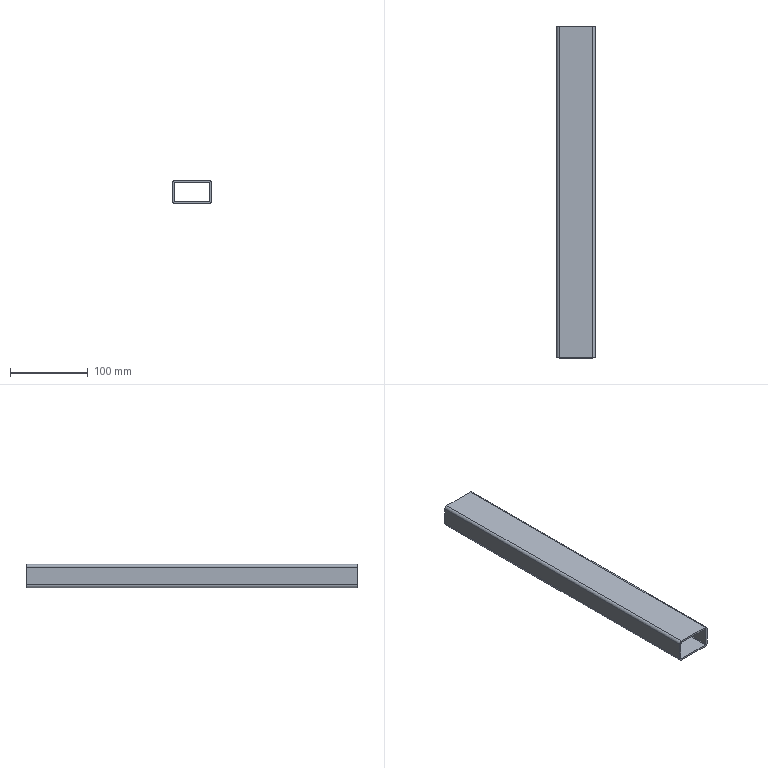Part | SolidWorks | features Extrusion 1 | 1 solid | 18 faces | box 50 x 428 x 30 mm | volume 144560 mm3 | plane 10 | cylinder 8 | commonest cylinder face diameters 2.3 x4 6.9 x4
STEP:
#1=CARTESIAN_POINT('',(25.,428.,-11.55));
#2=VERTEX_POINT('',#1);
#3=CARTESIAN_POINT('',(21.55,428.,-15.));
#4=VERTEX_POINT('',#3);
#5=CARTESIAN_POINT('',(21.55,428.,-11.55));
#6=DIRECTION('',(0.,1.,0.));
#7=DIRECTION('',(0.,0.,-1.));
#8=AXIS2_PLACEMENT_3D('',#5,#6,#7);
#9=CIRCLE('',#8,3.45);
#10=EDGE_CURVE('',#2,#4,#9,.T.);
#11=ORIENTED_EDGE('',*,*,#10,.T.);
#12=CARTESIAN_POINT('',(-21.55,428.,-15.));
#13=VERTEX_POINT('',#12);
#14=CARTESIAN_POINT('',(-21.55,428.,-15.));
#15=DIRECTION('',(-1.,0.,0.));
#16=VECTOR('',#15,1000.);
#17=LINE('',#14,#16);
#18=EDGE_CURVE('',#4,#13,#17,.T.);
#19=ORIENTED_EDGE('',*,*,#18,.T.);
#20=CARTESIAN_POINT('',(-25.,428.,-11.55));
#21=VERTEX_POINT('',#20);
#22=CARTESIAN_POINT('',(-21.55,428.,-11.55));
#23=DIRECTION('',(0.,1.,0.));
#24=DIRECTION('',(0.,0.,-1.));
#25=AXIS2_PLACEMENT_3D('',#22,#23,#24);
#26=CIRCLE('',#25,3.45);
#27=EDGE_CURVE('',#13,#21,#26,.T.);
#28=ORIENTED_EDGE('',*,*,#27,.T.);
#29=CARTESIAN_POINT('',(-25.,428.,11.55));
#30=VERTEX_POINT('',#29);
#31=CARTESIAN_POINT('',(-25.,428.,11.55));
#32=DIRECTION('',(0.,0.,1.));
#33=VECTOR('',#32,1000.);
#34=LINE('',#31,#33);
#35=EDGE_CURVE('',#21,#30,#34,.T.);
#36=ORIENTED_EDGE('',*,*,#35,.T.);
#37=CARTESIAN_POINT('',(-21.55,428.,15.));
#38=VERTEX_POINT('',#37);
#39=CARTESIAN_POINT('',(-21.55,428.,11.55));
#40=DIRECTION('',(0.,1.,0.));
#41=DIRECTION('',(0.,0.,-1.));
#42=AXIS2_PLACEMENT_3D('',#39,#40,#41);
#43=CIRCLE('',#42,3.45);
#44=EDGE_CURVE('',#30,#38,#43,.T.);
#45=ORIENTED_EDGE('',*,*,#44,.T.);
#46=CARTESIAN_POINT('',(21.55,428.,15.));
#47=VERTEX_POINT('',#46);
#48=CARTESIAN_POINT('',(-21.55,428.,15.));
#49=DIRECTION('',(1.,0.,0.));
#50=VECTOR('',#49,1000.);
#51=LINE('',#48,#50);
#52=EDGE_CURVE('',#38,#47,#51,.T.);
#53=ORIENTED_EDGE('',*,*,#52,.T.);
#54=CARTESIAN_POINT('',(25.,428.,11.55));
#55=VERTEX_POINT('',#54);
#56=CARTESIAN_POINT('',(21.55,428.,11.55));
#57=DIRECTION('',(0.,1.,0.));
#58=DIRECTION('',(0.,0.,1.));
#59=AXIS2_PLACEMENT_3D('',#56,#57,#58);
#60=CIRCLE('',#59,3.45);
#61=EDGE_CURVE('',#47,#55,#60,.T.);
#62=ORIENTED_EDGE('',*,*,#61,.T.);
#63=CARTESIAN_POINT('',(25.,428.,11.55));
#64=DIRECTION('',(0.,0.,-1.));
#65=VECTOR('',#64,1000.);
#66=LINE('',#63,#65);
#67=EDGE_CURVE('',#55,#2,#66,.T.);
#68=ORIENTED_EDGE('',*,*,#67,.T.);
#69=EDGE_LOOP('',(#11,#19,#28,#36,#45,#53,#62,#68));
#70=FACE_OUTER_BOUND('',#69,.T.);
#71=CARTESIAN_POINT('',(-22.7,428.,11.55));
#72=VERTEX_POINT('',#71);
#73=CARTESIAN_POINT('',(-21.55,428.,12.7));
#74=VERTEX_POINT('',#73);
#75=CARTESIAN_POINT('',(-21.55,428.,11.55));
#76=DIRECTION('',(0.,1.,0.));
#77=DIRECTION('',(0.,0.,-1.));
#78=AXIS2_PLACEMENT_3D('',#75,#76,#77);
#79=CIRCLE('',#78,1.15);
#80=EDGE_CURVE('',#72,#74,#79,.T.);
#81=ORIENTED_EDGE('',*,*,#80,.F.);
#82=CARTESIAN_POINT('',(-22.7,428.,-11.55));
#83=VERTEX_POINT('',#82);
#84=CARTESIAN_POINT('',(-22.7,428.,11.55));
#85=DIRECTION('',(0.,0.,1.));
#86=VECTOR('',#85,1000.);
#87=LINE('',#84,#86);
#88=EDGE_CURVE('',#83,#72,#87,.T.);
#89=ORIENTED_EDGE('',*,*,#88,.F.);
#90=CARTESIAN_POINT('',(-21.55,428.,-12.7));
#91=VERTEX_POINT('',#90);
#92=CARTESIAN_POINT('',(-21.55,428.,-11.55));
#93=DIRECTION('',(0.,1.,0.));
#94=DIRECTION('',(0.,0.,-1.));
#95=AXIS2_PLACEMENT_3D('',#92,#93,#94);
#96=CIRCLE('',#95,1.15);
#97=EDGE_CURVE('',#91,#83,#96,.T.);
#98=ORIENTED_EDGE('',*,*,#97,.F.);
#99=CARTESIAN_POINT('',(21.55,428.,-12.7));
#100=VERTEX_POINT('',#99);
#101=CARTESIAN_POINT('',(-21.55,428.,-12.7));
#102=DIRECTION('',(-1.,0.,0.));
#103=VECTOR('',#102,1000.);
#104=LINE('',#101,#103);
#105=EDGE_CURVE('',#100,#91,#104,.T.);
#106=ORIENTED_EDGE('',*,*,#105,.F.);
#107=CARTESIAN_POINT('',(22.7,428.,-11.55));
#108=VERTEX_POINT('',#107);
#109=CARTESIAN_POINT('',(21.55,428.,-11.55));
#110=DIRECTION('',(0.,1.,0.));
#111=DIRECTION('',(0.,0.,-1.));
#112=AXIS2_PLACEMENT_3D('',#109,#110,#111);
#113=CIRCLE('',#112,1.15);
#114=EDGE_CURVE('',#108,#100,#113,.T.);
#115=ORIENTED_EDGE('',*,*,#114,.F.);
#116=CARTESIAN_POINT('',(22.7,428.,11.55));
#117=VERTEX_POINT('',#116);
#118=CARTESIAN_POINT('',(22.7,428.,11.55));
#119=DIRECTION('',(0.,0.,-1.));
#120=VECTOR('',#119,1000.);
#121=LINE('',#118,#120);
#122=EDGE_CURVE('',#117,#108,#121,.T.);
#123=ORIENTED_EDGE('',*,*,#122,.F.);
#124=CARTESIAN_POINT('',(21.55,428.,12.7));
#125=VERTEX_POINT('',#124);
#126=CARTESIAN_POINT('',(21.55,428.,11.55));
#127=DIRECTION('',(0.,1.,0.));
#128=DIRECTION('',(0.,0.,1.));
#129=AXIS2_PLACEMENT_3D('',#126,#127,#128);
#130=CIRCLE('',#129,1.15);
#131=EDGE_CURVE('',#125,#117,#130,.T.);
#132=ORIENTED_EDGE('',*,*,#131,.F.);
#133=CARTESIAN_POINT('',(-21.55,428.,12.7));
#134=DIRECTION('',(1.,0.,0.));
#135=VECTOR('',#134,1000.);
#136=LINE('',#133,#135);
#137=EDGE_CURVE('',#74,#125,#136,.T.);
#138=ORIENTED_EDGE('',*,*,#137,.F.);
#139=EDGE_LOOP('',(#81,#89,#98,#106,#115,#123,#132,#138));
#140=FACE_BOUND('',#139,.T.);
#141=CARTESIAN_POINT('',(21.55,428.,-11.55));
#142=DIRECTION('',(0.,-1.,0.));
#143=DIRECTION('',(0.,0.,-1.));
#144=AXIS2_PLACEMENT_3D('',#141,#142,#143);
#145=PLANE('',#144);
#146=ADVANCED_FACE('',(#70,#140),#145,.F.);
#147=CARTESIAN_POINT('',(25.,0.,-11.55));
#148=VERTEX_POINT('',#147);
#149=CARTESIAN_POINT('',(21.55,0.,-15.));
#150=VERTEX_POINT('',#149);
#151=CARTESIAN_POINT('',(21.55,0.,-11.55));
#152=DIRECTION('',(0.,1.,0.));
#153=DIRECTION('',(0.,0.,-1.));
#154=AXIS2_PLACEMENT_3D('',#151,#152,#153);
#155=CIRCLE('',#154,3.45);
#156=EDGE_CURVE('',#148,#150,#155,.T.);
#157=ORIENTED_EDGE('',*,*,#156,.F.);
#158=CARTESIAN_POINT('',(25.,0.,11.55));
#159=VERTEX_POINT('',#158);
#160=CARTESIAN_POINT('',(25.,0.,11.55));
#161=DIRECTION('',(0.,0.,-1.));
#162=VECTOR('',#161,1000.);
#163=LINE('',#160,#162);
#164=EDGE_CURVE('',#159,#148,#163,.T.);
#165=ORIENTED_EDGE('',*,*,#164,.F.);
#166=CARTESIAN_POINT('',(21.55,0.,15.));
#167=VERTEX_POINT('',#166);
#168=CARTESIAN_POINT('',(21.55,0.,11.55));
#169=DIRECTION('',(0.,1.,0.));
#170=DIRECTION('',(0.,0.,1.));
#171=AXIS2_PLACEMENT_3D('',#168,#169,#170);
#172=CIRCLE('',#171,3.45);
#173=EDGE_CURVE('',#167,#159,#172,.T.);
#174=ORIENTED_EDGE('',*,*,#173,.F.);
#175=CARTESIAN_POINT('',(-21.55,0.,15.));
#176=VERTEX_POINT('',#175);
#177=CARTESIAN_POINT('',(-21.55,0.,15.));
#178=DIRECTION('',(1.,0.,0.));
#179=VECTOR('',#178,1000.);
#180=LINE('',#177,#179);
#181=EDGE_CURVE('',#176,#167,#180,.T.);
#182=ORIENTED_EDGE('',*,*,#181,.F.);
#183=CARTESIAN_POINT('',(-25.,0.,11.55));
#184=VERTEX_POINT('',#183);
#185=CARTESIAN_POINT('',(-21.55,0.,11.55));
#186=DIRECTION('',(0.,1.,0.));
#187=DIRECTION('',(0.,0.,-1.));
#188=AXIS2_PLACEMENT_3D('',#185,#186,#187);
#189=CIRCLE('',#188,3.45);
#190=EDGE_CURVE('',#184,#176,#189,.T.);
#191=ORIENTED_EDGE('',*,*,#190,.F.);
#192=CARTESIAN_POINT('',(-25.,0.,-11.55));
#193=VERTEX_POINT('',#192);
#194=CARTESIAN_POINT('',(-25.,0.,11.55));
#195=DIRECTION('',(0.,0.,1.));
#196=VECTOR('',#195,1000.);
#197=LINE('',#194,#196);
#198=EDGE_CURVE('',#193,#184,#197,.T.);
#199=ORIENTED_EDGE('',*,*,#198,.F.);
#200=CARTESIAN_POINT('',(-21.55,0.,-15.));
#201=VERTEX_POINT('',#200);
#202=CARTESIAN_POINT('',(-21.55,0.,-11.55));
#203=DIRECTION('',(0.,1.,0.));
#204=DIRECTION('',(0.,0.,-1.));
#205=AXIS2_PLACEMENT_3D('',#202,#203,#204);
#206=CIRCLE('',#205,3.45);
#207=EDGE_CURVE('',#201,#193,#206,.T.);
#208=ORIENTED_EDGE('',*,*,#207,.F.);
#209=CARTESIAN_POINT('',(-21.55,0.,-15.));
#210=DIRECTION('',(-1.,0.,0.));
#211=VECTOR('',#210,1000.);
#212=LINE('',#209,#211);
#213=EDGE_CURVE('',#150,#201,#212,.T.);
#214=ORIENTED_EDGE('',*,*,#213,.F.);
#215=EDGE_LOOP('',(#157,#165,#174,#182,#191,#199,#208,#214));
#216=FACE_OUTER_BOUND('',#215,.T.);
#217=CARTESIAN_POINT('',(-22.7,0.,-11.55));
#218=VERTEX_POINT('',#217);
#219=CARTESIAN_POINT('',(-22.7,0.,11.55));
#220=VERTEX_POINT('',#219);
#221=CARTESIAN_POINT('',(-22.7,0.,11.55));
#222=DIRECTION('',(0.,0.,1.));
#223=VECTOR('',#222,1000.);
#224=LINE('',#221,#223);
#225=EDGE_CURVE('',#218,#220,#224,.T.);
#226=ORIENTED_EDGE('',*,*,#225,.T.);
#227=CARTESIAN_POINT('',(-21.55,0.,12.7));
#228=VERTEX_POINT('',#227);
#229=CARTESIAN_POINT('',(-21.55,0.,11.55));
#230=DIRECTION('',(0.,1.,0.));
#231=DIRECTION('',(0.,0.,-1.));
#232=AXIS2_PLACEMENT_3D('',#229,#230,#231);
#233=CIRCLE('',#232,1.15);
#234=EDGE_CURVE('',#220,#228,#233,.T.);
#235=ORIENTED_EDGE('',*,*,#234,.T.);
#236=CARTESIAN_POINT('',(21.55,0.,12.7));
#237=VERTEX_POINT('',#236);
#238=CARTESIAN_POINT('',(-21.55,0.,12.7));
#239=DIRECTION('',(1.,0.,0.));
#240=VECTOR('',#239,1000.);
#241=LINE('',#238,#240);
#242=EDGE_CURVE('',#228,#237,#241,.T.);
#243=ORIENTED_EDGE('',*,*,#242,.T.);
#244=CARTESIAN_POINT('',(22.7,0.,11.55));
#245=VERTEX_POINT('',#244);
#246=CARTESIAN_POINT('',(21.55,0.,11.55));
#247=DIRECTION('',(0.,1.,0.));
#248=DIRECTION('',(0.,0.,1.));
#249=AXIS2_PLACEMENT_3D('',#246,#247,#248);
#250=CIRCLE('',#249,1.15);
#251=EDGE_CURVE('',#237,#245,#250,.T.);
#252=ORIENTED_EDGE('',*,*,#251,.T.);
#253=CARTESIAN_POINT('',(22.7,0.,-11.55));
#254=VERTEX_POINT('',#253);
#255=CARTESIAN_POINT('',(22.7,0.,11.55));
#256=DIRECTION('',(0.,0.,-1.));
#257=VECTOR('',#256,1000.);
#258=LINE('',#255,#257);
#259=EDGE_CURVE('',#245,#254,#258,.T.);
#260=ORIENTED_EDGE('',*,*,#259,.T.);
#261=CARTESIAN_POINT('',(21.55,0.,-12.7));
#262=VERTEX_POINT('',#261);
#263=CARTESIAN_POINT('',(21.55,0.,-11.55));
#264=DIRECTION('',(0.,1.,0.));
#265=DIRECTION('',(0.,0.,-1.));
#266=AXIS2_PLACEMENT_3D('',#263,#264,#265);
#267=CIRCLE('',#266,1.15);
#268=EDGE_CURVE('',#254,#262,#267,.T.);
#269=ORIENTED_EDGE('',*,*,#268,.T.);
#270=CARTESIAN_POINT('',(-21.55,0.,-12.7));
#271=VERTEX_POINT('',#270);
#272=CARTESIAN_POINT('',(-21.55,0.,-12.7));
#273=DIRECTION('',(-1.,0.,0.));
#274=VECTOR('',#273,1000.);
#275=LINE('',#272,#274);
#276=EDGE_CURVE('',#262,#271,#275,.T.);
#277=ORIENTED_EDGE('',*,*,#276,.T.);
#278=CARTESIAN_POINT('',(-21.55,0.,-11.55));
#279=DIRECTION('',(0.,1.,0.));
#280=DIRECTION('',(0.,0.,-1.));
#281=AXIS2_PLACEMENT_3D('',#278,#279,#280);
#282=CIRCLE('',#281,1.15);
#283=EDGE_CURVE('',#271,#218,#282,.T.);
#284=ORIENTED_EDGE('',*,*,#283,.T.);
#285=EDGE_LOOP('',(#226,#235,#243,#252,#260,#269,#277,#284));
#286=FACE_BOUND('',#285,.T.);
#287=CARTESIAN_POINT('',(21.55,0.,-11.55));
#288=DIRECTION('',(0.,-1.,0.));
#289=DIRECTION('',(0.,0.,-1.));
#290=AXIS2_PLACEMENT_3D('',#287,#288,#289);
#291=PLANE('',#290);
#292=ADVANCED_FACE('',(#216,#286),#291,.T.);
#293=ORIENTED_EDGE('',*,*,#156,.T.);
#294=CARTESIAN_POINT('',(21.55,428.,-15.));
#295=DIRECTION('',(0.,-1.,0.));
#296=VECTOR('',#295,1000.);
#297=LINE('',#294,#296);
#298=EDGE_CURVE('',#4,#150,#297,.T.);
#299=ORIENTED_EDGE('',*,*,#298,.F.);
#300=ORIENTED_EDGE('',*,*,#10,.F.);
#301=CARTESIAN_POINT('',(25.,428.,-11.55));
#302=DIRECTION('',(0.,-1.,0.));
#303=VECTOR('',#302,1000.);
#304=LINE('',#301,#303);
#305=EDGE_CURVE('',#2,#148,#304,.T.);
#306=ORIENTED_EDGE('',*,*,#305,.T.);
#307=EDGE_LOOP('',(#293,#299,#300,#306));
#308=FACE_OUTER_BOUND('',#307,.T.);
#309=CARTESIAN_POINT('',(21.55,428.,-11.55));
#310=DIRECTION('',(0.,-1.,0.));
#311=DIRECTION('',(0.,0.,-1.));
#312=AXIS2_PLACEMENT_3D('',#309,#310,#311);
#313=CYLINDRICAL_SURFACE('',#312,3.45);
#314=ADVANCED_FACE('',(#308),#313,.T.);
#315=ORIENTED_EDGE('',*,*,#213,.T.);
#316=CARTESIAN_POINT('',(-21.55,428.,-15.));
#317=DIRECTION('',(0.,-1.,0.));
#318=VECTOR('',#317,1000.);
#319=LINE('',#316,#318);
#320=EDGE_CURVE('',#13,#201,#319,.T.);
#321=ORIENTED_EDGE('',*,*,#320,.F.);
#322=ORIENTED_EDGE('',*,*,#18,.F.);
#323=ORIENTED_EDGE('',*,*,#298,.T.);
#324=EDGE_LOOP('',(#315,#321,#322,#323));
#325=FACE_OUTER_BOUND('',#324,.T.);
#326=CARTESIAN_POINT('',(-21.55,428.,-15.));
#327=DIRECTION('',(0.,0.,1.));
#328=DIRECTION('',(1.,0.,0.));
#329=AXIS2_PLACEMENT_3D('',#326,#327,#328);
#330=PLANE('',#329);
#331=ADVANCED_FACE('',(#325),#330,.F.);
#332=ORIENTED_EDGE('',*,*,#207,.T.);
#333=CARTESIAN_POINT('',(-25.,428.,-11.55));
#334=DIRECTION('',(0.,-1.,0.));
#335=VECTOR('',#334,1000.);
#336=LINE('',#333,#335);
#337=EDGE_CURVE('',#21,#193,#336,.T.);
#338=ORIENTED_EDGE('',*,*,#337,.F.);
#339=ORIENTED_EDGE('',*,*,#27,.F.);
#340=ORIENTED_EDGE('',*,*,#320,.T.);
#341=EDGE_LOOP('',(#332,#338,#339,#340));
#342=FACE_OUTER_BOUND('',#341,.T.);
#343=CARTESIAN_POINT('',(-21.55,428.,-11.55));
#344=DIRECTION('',(0.,-1.,0.));
#345=DIRECTION('',(0.,0.,-1.));
#346=AXIS2_PLACEMENT_3D('',#343,#344,#345);
#347=CYLINDRICAL_SURFACE('',#346,3.45);
#348=ADVANCED_FACE('',(#342),#347,.T.);
#349=ORIENTED_EDGE('',*,*,#198,.T.);
#350=CARTESIAN_POINT('',(-25.,428.,11.55));
#351=DIRECTION('',(0.,-1.,0.));
#352=VECTOR('',#351,1000.);
#353=LINE('',#350,#352);
#354=EDGE_CURVE('',#30,#184,#353,.T.);
#355=ORIENTED_EDGE('',*,*,#354,.F.);
#356=ORIENTED_EDGE('',*,*,#35,.F.);
#357=ORIENTED_EDGE('',*,*,#337,.T.);
#358=EDGE_LOOP('',(#349,#355,#356,#357));
#359=FACE_OUTER_BOUND('',#358,.T.);
#360=CARTESIAN_POINT('',(-25.,428.,11.55));
#361=DIRECTION('',(1.,0.,0.));
#362=DIRECTION('',(0.,0.,-1.));
#363=AXIS2_PLACEMENT_3D('',#360,#361,#362);
#364=PLANE('',#363);
#365=ADVANCED_FACE('',(#359),#364,.F.);
#366=ORIENTED_EDGE('',*,*,#190,.T.);
#367=CARTESIAN_POINT('',(-21.55,428.,15.));
#368=DIRECTION('',(0.,-1.,0.));
#369=VECTOR('',#368,1000.);
#370=LINE('',#367,#369);
#371=EDGE_CURVE('',#38,#176,#370,.T.);
#372=ORIENTED_EDGE('',*,*,#371,.F.);
#373=ORIENTED_EDGE('',*,*,#44,.F.);
#374=ORIENTED_EDGE('',*,*,#354,.T.);
#375=EDGE_LOOP('',(#366,#372,#373,#374));
#376=FACE_OUTER_BOUND('',#375,.T.);
#377=CARTESIAN_POINT('',(-21.55,428.,11.55));
#378=DIRECTION('',(0.,-1.,0.));
#379=DIRECTION('',(0.,0.,-1.));
#380=AXIS2_PLACEMENT_3D('',#377,#378,#379);
#381=CYLINDRICAL_SURFACE('',#380,3.45);
#382=ADVANCED_FACE('',(#376),#381,.T.);
#383=ORIENTED_EDGE('',*,*,#181,.T.);
#384=CARTESIAN_POINT('',(21.55,428.,15.));
#385=DIRECTION('',(0.,-1.,0.));
#386=VECTOR('',#385,1000.);
#387=LINE('',#384,#386);
#388=EDGE_CURVE('',#47,#167,#387,.T.);
#389=ORIENTED_EDGE('',*,*,#388,.F.);
#390=ORIENTED_EDGE('',*,*,#52,.F.);
#391=ORIENTED_EDGE('',*,*,#371,.T.);
#392=EDGE_LOOP('',(#383,#389,#390,#391));
#393=FACE_OUTER_BOUND('',#392,.T.);
#394=CARTESIAN_POINT('',(-21.55,428.,15.));
#395=DIRECTION('',(0.,0.,-1.));
#396=DIRECTION('',(-1.,0.,0.));
#397=AXIS2_PLACEMENT_3D('',#394,#395,#396);
#398=PLANE('',#397);
#399=ADVANCED_FACE('',(#393),#398,.F.);
#400=ORIENTED_EDGE('',*,*,#173,.T.);
#401=CARTESIAN_POINT('',(25.,428.,11.55));
#402=DIRECTION('',(0.,-1.,0.));
#403=VECTOR('',#402,1000.);
#404=LINE('',#401,#403);
#405=EDGE_CURVE('',#55,#159,#404,.T.);
#406=ORIENTED_EDGE('',*,*,#405,.F.);
#407=ORIENTED_EDGE('',*,*,#61,.F.);
#408=ORIENTED_EDGE('',*,*,#388,.T.);
#409=EDGE_LOOP('',(#400,#406,#407,#408));
#410=FACE_OUTER_BOUND('',#409,.T.);
#411=CARTESIAN_POINT('',(21.55,428.,11.55));
#412=DIRECTION('',(0.,-1.,0.));
#413=DIRECTION('',(0.,0.,-1.));
#414=AXIS2_PLACEMENT_3D('',#411,#412,#413);
#415=CYLINDRICAL_SURFACE('',#414,3.45);
#416=ADVANCED_FACE('',(#410),#415,.T.);
#417=ORIENTED_EDGE('',*,*,#164,.T.);
#418=ORIENTED_EDGE('',*,*,#305,.F.);
#419=ORIENTED_EDGE('',*,*,#67,.F.);
#420=ORIENTED_EDGE('',*,*,#405,.T.);
#421=EDGE_LOOP('',(#417,#418,#419,#420));
#422=FACE_OUTER_BOUND('',#421,.T.);
#423=CARTESIAN_POINT('',(25.,428.,11.55));
#424=DIRECTION('',(-1.,0.,0.));
#425=DIRECTION('',(0.,0.,1.));
#426=AXIS2_PLACEMENT_3D('',#423,#424,#425);
#427=PLANE('',#426);
#428=ADVANCED_FACE('',(#422),#427,.F.);
#429=ORIENTED_EDGE('',*,*,#234,.F.);
#430=CARTESIAN_POINT('',(-22.7,428.,11.55));
#431=DIRECTION('',(0.,-1.,0.));
#432=VECTOR('',#431,1000.);
#433=LINE('',#430,#432);
#434=EDGE_CURVE('',#72,#220,#433,.T.);
#435=ORIENTED_EDGE('',*,*,#434,.F.);
#436=ORIENTED_EDGE('',*,*,#80,.T.);
#437=CARTESIAN_POINT('',(-21.55,428.,12.7));
#438=DIRECTION('',(0.,-1.,0.));
#439=VECTOR('',#438,1000.);
#440=LINE('',#437,#439);
#441=EDGE_CURVE('',#74,#228,#440,.T.);
#442=ORIENTED_EDGE('',*,*,#441,.T.);
#443=EDGE_LOOP('',(#429,#435,#436,#442));
#444=FACE_OUTER_BOUND('',#443,.T.);
#445=CARTESIAN_POINT('',(-21.55,428.,11.55));
#446=DIRECTION('',(0.,-1.,0.));
#447=DIRECTION('',(0.,0.,-1.));
#448=AXIS2_PLACEMENT_3D('',#445,#446,#447);
#449=CYLINDRICAL_SURFACE('',#448,1.15);
#450=ADVANCED_FACE('',(#444),#449,.F.);
#451=ORIENTED_EDGE('',*,*,#242,.F.);
#452=ORIENTED_EDGE('',*,*,#441,.F.);
#453=ORIENTED_EDGE('',*,*,#137,.T.);
#454=CARTESIAN_POINT('',(21.55,428.,12.7));
#455=DIRECTION('',(0.,-1.,0.));
#456=VECTOR('',#455,1000.);
#457=LINE('',#454,#456);
#458=EDGE_CURVE('',#125,#237,#457,.T.);
#459=ORIENTED_EDGE('',*,*,#458,.T.);
#460=EDGE_LOOP('',(#451,#452,#453,#459));
#461=FACE_OUTER_BOUND('',#460,.T.);
#462=CARTESIAN_POINT('',(-21.55,428.,12.7));
#463=DIRECTION('',(0.,0.,-1.));
#464=DIRECTION('',(-1.,0.,0.));
#465=AXIS2_PLACEMENT_3D('',#462,#463,#464);
#466=PLANE('',#465);
#467=ADVANCED_FACE('',(#461),#466,.T.);
#468=ORIENTED_EDGE('',*,*,#251,.F.);
#469=ORIENTED_EDGE('',*,*,#458,.F.);
#470=ORIENTED_EDGE('',*,*,#131,.T.);
#471=CARTESIAN_POINT('',(22.7,428.,11.55));
#472=DIRECTION('',(0.,-1.,0.));
#473=VECTOR('',#472,1000.);
#474=LINE('',#471,#473);
#475=EDGE_CURVE('',#117,#245,#474,.T.);
#476=ORIENTED_EDGE('',*,*,#475,.T.);
#477=EDGE_LOOP('',(#468,#469,#470,#476));
#478=FACE_OUTER_BOUND('',#477,.T.);
#479=CARTESIAN_POINT('',(21.55,428.,11.55));
#480=DIRECTION('',(0.,-1.,0.));
#481=DIRECTION('',(0.,0.,-1.));
#482=AXIS2_PLACEMENT_3D('',#479,#480,#481);
#483=CYLINDRICAL_SURFACE('',#482,1.15);
#484=ADVANCED_FACE('',(#478),#483,.F.);
#485=ORIENTED_EDGE('',*,*,#259,.F.);
#486=ORIENTED_EDGE('',*,*,#475,.F.);
#487=ORIENTED_EDGE('',*,*,#122,.T.);
#488=CARTESIAN_POINT('',(22.7,428.,-11.55));
#489=DIRECTION('',(0.,-1.,0.));
#490=VECTOR('',#489,1000.);
#491=LINE('',#488,#490);
#492=EDGE_CURVE('',#108,#254,#491,.T.);
#493=ORIENTED_EDGE('',*,*,#492,.T.);
#494=EDGE_LOOP('',(#485,#486,#487,#493));
#495=FACE_OUTER_BOUND('',#494,.T.);
#496=CARTESIAN_POINT('',(22.7,428.,11.55));
#497=DIRECTION('',(-1.,0.,0.));
#498=DIRECTION('',(0.,0.,1.));
#499=AXIS2_PLACEMENT_3D('',#496,#497,#498);
#500=PLANE('',#499);
#501=ADVANCED_FACE('',(#495),#500,.T.);
#502=ORIENTED_EDGE('',*,*,#268,.F.);
#503=ORIENTED_EDGE('',*,*,#492,.F.);
#504=ORIENTED_EDGE('',*,*,#114,.T.);
#505=CARTESIAN_POINT('',(21.55,428.,-12.7));
#506=DIRECTION('',(0.,-1.,0.));
#507=VECTOR('',#506,1000.);
#508=LINE('',#505,#507);
#509=EDGE_CURVE('',#100,#262,#508,.T.);
#510=ORIENTED_EDGE('',*,*,#509,.T.);
#511=EDGE_LOOP('',(#502,#503,#504,#510));
#512=FACE_OUTER_BOUND('',#511,.T.);
#513=CARTESIAN_POINT('',(21.55,428.,-11.55));
#514=DIRECTION('',(0.,-1.,0.));
#515=DIRECTION('',(0.,0.,-1.));
#516=AXIS2_PLACEMENT_3D('',#513,#514,#515);
#517=CYLINDRICAL_SURFACE('',#516,1.15);
#518=ADVANCED_FACE('',(#512),#517,.F.);
#519=ORIENTED_EDGE('',*,*,#276,.F.);
#520=ORIENTED_EDGE('',*,*,#509,.F.);
#521=ORIENTED_EDGE('',*,*,#105,.T.);
#522=CARTESIAN_POINT('',(-21.55,428.,-12.7));
#523=DIRECTION('',(0.,-1.,0.));
#524=VECTOR('',#523,1000.);
#525=LINE('',#522,#524);
#526=EDGE_CURVE('',#91,#271,#525,.T.);
#527=ORIENTED_EDGE('',*,*,#526,.T.);
#528=EDGE_LOOP('',(#519,#520,#521,#527));
#529=FACE_OUTER_BOUND('',#528,.T.);
#530=CARTESIAN_POINT('',(-21.55,428.,-12.7));
#531=DIRECTION('',(0.,0.,1.));
#532=DIRECTION('',(1.,0.,0.));
#533=AXIS2_PLACEMENT_3D('',#530,#531,#532);
#534=PLANE('',#533);
#535=ADVANCED_FACE('',(#529),#534,.T.);
#536=ORIENTED_EDGE('',*,*,#283,.F.);
#537=ORIENTED_EDGE('',*,*,#526,.F.);
#538=ORIENTED_EDGE('',*,*,#97,.T.);
#539=CARTESIAN_POINT('',(-22.7,428.,-11.55));
#540=DIRECTION('',(0.,-1.,0.));
#541=VECTOR('',#540,1000.);
#542=LINE('',#539,#541);
#543=EDGE_CURVE('',#83,#218,#542,.T.);
#544=ORIENTED_EDGE('',*,*,#543,.T.);
#545=EDGE_LOOP('',(#536,#537,#538,#544));
#546=FACE_OUTER_BOUND('',#545,.T.);
#547=CARTESIAN_POINT('',(-21.55,428.,-11.55));
#548=DIRECTION('',(0.,-1.,0.));
#549=DIRECTION('',(0.,0.,-1.));
#550=AXIS2_PLACEMENT_3D('',#547,#548,#549);
#551=CYLINDRICAL_SURFACE('',#550,1.15);
#552=ADVANCED_FACE('',(#546),#551,.F.);
#553=ORIENTED_EDGE('',*,*,#225,.F.);
#554=ORIENTED_EDGE('',*,*,#543,.F.);
#555=ORIENTED_EDGE('',*,*,#88,.T.);
#556=ORIENTED_EDGE('',*,*,#434,.T.);
#557=EDGE_LOOP('',(#553,#554,#555,#556));
#558=FACE_OUTER_BOUND('',#557,.T.);
#559=CARTESIAN_POINT('',(-22.7,428.,11.55));
#560=DIRECTION('',(1.,0.,0.));
#561=DIRECTION('',(0.,0.,-1.));
#562=AXIS2_PLACEMENT_3D('',#559,#560,#561);
#563=PLANE('',#562);
#564=ADVANCED_FACE('',(#558),#563,.T.);
#565=CLOSED_SHELL('',(#146,#292,#314,#331,#348,#365,#382,#399,#416,#428,#450,#467,#484,#501,#518,#535,#552,#564));
#566=MANIFOLD_SOLID_BREP('',#565);
#567=CARTESIAN_POINT('',(0.,0.,0.));
#568=DIRECTION('',(0.,0.,1.));
#569=DIRECTION('',(1.,0.,0.));
#570=AXIS2_PLACEMENT_3D('',#567,#568,#569);
#571=(LENGTH_UNIT()NAMED_UNIT(*)SI_UNIT(.MILLI.,.METRE.));
#572=UNCERTAINTY_MEASURE_WITH_UNIT(LENGTH_MEASURE(0.00001),#571,'','');
#573=(NAMED_UNIT(*)PLANE_ANGLE_UNIT()SI_UNIT($,.RADIAN.));
#574=(NAMED_UNIT(*)SI_UNIT($,.STERADIAN.)SOLID_ANGLE_UNIT());
#575=(GEOMETRIC_REPRESENTATION_CONTEXT(3)GLOBAL_UNCERTAINTY_ASSIGNED_CONTEXT((#572))GLOBAL_UNIT_ASSIGNED_CONTEXT((#571,#573,#574))REPRESENTATION_CONTEXT('',''));
#576=ADVANCED_BREP_SHAPE_REPRESENTATION('',(#566,#570),#575);